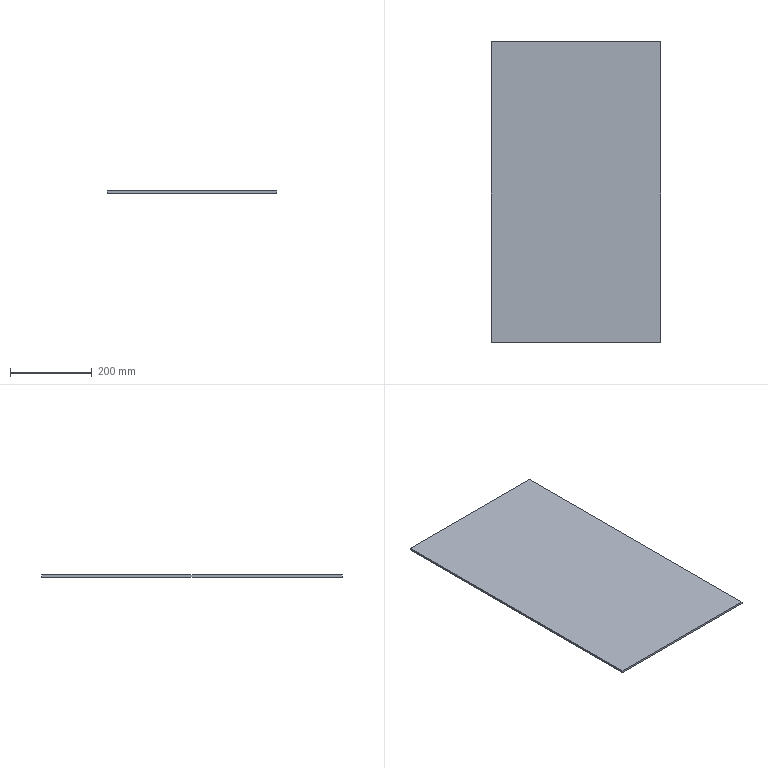Part | SolidWorks | features Extrusion 1, HoleWzd 1 | 1 solid | 6 faces | box 414 x 736 x 5 mm | volume 1523520 mm3 | plane 6
STEP:
#1=CARTESIAN_POINT('',(207.,-368.,0.));
#2=VERTEX_POINT('',#1);
#3=CARTESIAN_POINT('',(207.,368.,0.));
#4=VERTEX_POINT('',#3);
#5=CARTESIAN_POINT('',(207.,368.,0.));
#6=DIRECTION('',(0.,1.,0.));
#7=VECTOR('',#6,1000.);
#8=LINE('',#5,#7);
#9=EDGE_CURVE('',#2,#4,#8,.T.);
#10=ORIENTED_EDGE('',*,*,#9,.T.);
#11=CARTESIAN_POINT('',(207.,368.,5.));
#12=VERTEX_POINT('',#11);
#13=CARTESIAN_POINT('',(207.,368.,5.));
#14=DIRECTION('',(0.,0.,-1.));
#15=VECTOR('',#14,1000.);
#16=LINE('',#13,#15);
#17=EDGE_CURVE('',#12,#4,#16,.T.);
#18=ORIENTED_EDGE('',*,*,#17,.F.);
#19=CARTESIAN_POINT('',(207.,-368.,5.));
#20=VERTEX_POINT('',#19);
#21=CARTESIAN_POINT('',(207.,368.,5.));
#22=DIRECTION('',(0.,1.,0.));
#23=VECTOR('',#22,1000.);
#24=LINE('',#21,#23);
#25=EDGE_CURVE('',#20,#12,#24,.T.);
#26=ORIENTED_EDGE('',*,*,#25,.F.);
#27=CARTESIAN_POINT('',(207.,-368.,5.));
#28=DIRECTION('',(0.,0.,-1.));
#29=VECTOR('',#28,1000.);
#30=LINE('',#27,#29);
#31=EDGE_CURVE('',#20,#2,#30,.T.);
#32=ORIENTED_EDGE('',*,*,#31,.T.);
#33=EDGE_LOOP('',(#10,#18,#26,#32));
#34=FACE_OUTER_BOUND('',#33,.T.);
#35=CARTESIAN_POINT('',(207.,368.,5.));
#36=DIRECTION('',(-1.,0.,0.));
#37=DIRECTION('',(0.,-1.,0.));
#38=AXIS2_PLACEMENT_3D('',#35,#36,#37);
#39=PLANE('',#38);
#40=ADVANCED_FACE('',(#34),#39,.F.);
#41=CARTESIAN_POINT('',(-207.,368.,0.));
#42=VERTEX_POINT('',#41);
#43=CARTESIAN_POINT('',(-207.,368.,0.));
#44=DIRECTION('',(-1.,0.,0.));
#45=VECTOR('',#44,1000.);
#46=LINE('',#43,#45);
#47=EDGE_CURVE('',#4,#42,#46,.T.);
#48=ORIENTED_EDGE('',*,*,#47,.T.);
#49=CARTESIAN_POINT('',(-207.,368.,5.));
#50=VERTEX_POINT('',#49);
#51=CARTESIAN_POINT('',(-207.,368.,5.));
#52=DIRECTION('',(0.,0.,-1.));
#53=VECTOR('',#52,1000.);
#54=LINE('',#51,#53);
#55=EDGE_CURVE('',#50,#42,#54,.T.);
#56=ORIENTED_EDGE('',*,*,#55,.F.);
#57=CARTESIAN_POINT('',(-207.,368.,5.));
#58=DIRECTION('',(-1.,0.,0.));
#59=VECTOR('',#58,1000.);
#60=LINE('',#57,#59);
#61=EDGE_CURVE('',#12,#50,#60,.T.);
#62=ORIENTED_EDGE('',*,*,#61,.F.);
#63=ORIENTED_EDGE('',*,*,#17,.T.);
#64=EDGE_LOOP('',(#48,#56,#62,#63));
#65=FACE_OUTER_BOUND('',#64,.T.);
#66=CARTESIAN_POINT('',(-207.,368.,5.));
#67=DIRECTION('',(0.,-1.,0.));
#68=DIRECTION('',(0.,0.,-1.));
#69=AXIS2_PLACEMENT_3D('',#66,#67,#68);
#70=PLANE('',#69);
#71=ADVANCED_FACE('',(#65),#70,.F.);
#72=CARTESIAN_POINT('',(-207.,-368.,0.));
#73=VERTEX_POINT('',#72);
#74=CARTESIAN_POINT('',(-207.,368.,0.));
#75=DIRECTION('',(0.,-1.,0.));
#76=VECTOR('',#75,1000.);
#77=LINE('',#74,#76);
#78=EDGE_CURVE('',#42,#73,#77,.T.);
#79=ORIENTED_EDGE('',*,*,#78,.T.);
#80=CARTESIAN_POINT('',(-207.,-368.,5.));
#81=VERTEX_POINT('',#80);
#82=CARTESIAN_POINT('',(-207.,-368.,5.));
#83=DIRECTION('',(0.,0.,-1.));
#84=VECTOR('',#83,1000.);
#85=LINE('',#82,#84);
#86=EDGE_CURVE('',#81,#73,#85,.T.);
#87=ORIENTED_EDGE('',*,*,#86,.F.);
#88=CARTESIAN_POINT('',(-207.,368.,5.));
#89=DIRECTION('',(0.,-1.,0.));
#90=VECTOR('',#89,1000.);
#91=LINE('',#88,#90);
#92=EDGE_CURVE('',#50,#81,#91,.T.);
#93=ORIENTED_EDGE('',*,*,#92,.F.);
#94=ORIENTED_EDGE('',*,*,#55,.T.);
#95=EDGE_LOOP('',(#79,#87,#93,#94));
#96=FACE_OUTER_BOUND('',#95,.T.);
#97=CARTESIAN_POINT('',(-207.,368.,5.));
#98=DIRECTION('',(1.,0.,0.));
#99=DIRECTION('',(0.,1.,0.));
#100=AXIS2_PLACEMENT_3D('',#97,#98,#99);
#101=PLANE('',#100);
#102=ADVANCED_FACE('',(#96),#101,.F.);
#103=CARTESIAN_POINT('',(-207.,-368.,0.));
#104=DIRECTION('',(1.,0.,0.));
#105=VECTOR('',#104,1000.);
#106=LINE('',#103,#105);
#107=EDGE_CURVE('',#73,#2,#106,.T.);
#108=ORIENTED_EDGE('',*,*,#107,.T.);
#109=ORIENTED_EDGE('',*,*,#31,.F.);
#110=CARTESIAN_POINT('',(-207.,-368.,5.));
#111=DIRECTION('',(1.,0.,0.));
#112=VECTOR('',#111,1000.);
#113=LINE('',#110,#112);
#114=EDGE_CURVE('',#81,#20,#113,.T.);
#115=ORIENTED_EDGE('',*,*,#114,.F.);
#116=ORIENTED_EDGE('',*,*,#86,.T.);
#117=EDGE_LOOP('',(#108,#109,#115,#116));
#118=FACE_OUTER_BOUND('',#117,.T.);
#119=CARTESIAN_POINT('',(-207.,-368.,5.));
#120=DIRECTION('',(0.,1.,0.));
#121=DIRECTION('',(0.,0.,1.));
#122=AXIS2_PLACEMENT_3D('',#119,#120,#121);
#123=PLANE('',#122);
#124=ADVANCED_FACE('',(#118),#123,.F.);
#125=ORIENTED_EDGE('',*,*,#25,.T.);
#126=ORIENTED_EDGE('',*,*,#61,.T.);
#127=ORIENTED_EDGE('',*,*,#92,.T.);
#128=ORIENTED_EDGE('',*,*,#114,.T.);
#129=EDGE_LOOP('',(#125,#126,#127,#128));
#130=FACE_OUTER_BOUND('',#129,.T.);
#131=CARTESIAN_POINT('',(0.,0.,5.));
#132=DIRECTION('',(0.,0.,1.));
#133=DIRECTION('',(1.,0.,0.));
#134=AXIS2_PLACEMENT_3D('',#131,#132,#133);
#135=PLANE('',#134);
#136=ADVANCED_FACE('',(#130),#135,.T.);
#137=ORIENTED_EDGE('',*,*,#9,.F.);
#138=ORIENTED_EDGE('',*,*,#107,.F.);
#139=ORIENTED_EDGE('',*,*,#78,.F.);
#140=ORIENTED_EDGE('',*,*,#47,.F.);
#141=EDGE_LOOP('',(#137,#138,#139,#140));
#142=FACE_OUTER_BOUND('',#141,.T.);
#143=CARTESIAN_POINT('',(0.,0.,0.));
#144=DIRECTION('',(0.,0.,1.));
#145=DIRECTION('',(1.,0.,0.));
#146=AXIS2_PLACEMENT_3D('',#143,#144,#145);
#147=PLANE('',#146);
#148=ADVANCED_FACE('',(#142),#147,.F.);
#149=CLOSED_SHELL('',(#40,#71,#102,#124,#136,#148));
#150=MANIFOLD_SOLID_BREP('',#149);
#151=CARTESIAN_POINT('',(0.,0.,0.));
#152=DIRECTION('',(0.,0.,1.));
#153=DIRECTION('',(1.,0.,0.));
#154=AXIS2_PLACEMENT_3D('',#151,#152,#153);
#155=(LENGTH_UNIT()NAMED_UNIT(*)SI_UNIT(.MILLI.,.METRE.));
#156=UNCERTAINTY_MEASURE_WITH_UNIT(LENGTH_MEASURE(0.00001),#155,'','');
#157=(NAMED_UNIT(*)PLANE_ANGLE_UNIT()SI_UNIT($,.RADIAN.));
#158=(NAMED_UNIT(*)SI_UNIT($,.STERADIAN.)SOLID_ANGLE_UNIT());
#159=(GEOMETRIC_REPRESENTATION_CONTEXT(3)GLOBAL_UNCERTAINTY_ASSIGNED_CONTEXT((#156))GLOBAL_UNIT_ASSIGNED_CONTEXT((#155,#157,#158))REPRESENTATION_CONTEXT('',''));
#160=ADVANCED_BREP_SHAPE_REPRESENTATION('',(#150,#154),#159);